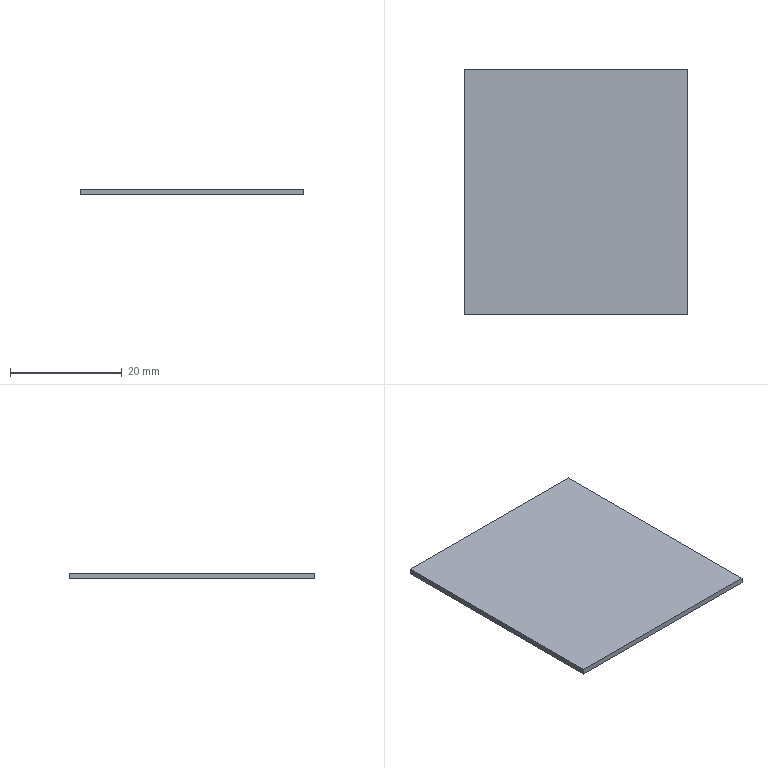Part | SolidWorks | features BaseBody 1 | 1 solid | 6 faces | box 40 x 44 x 1 mm | volume 1760 mm3 | plane 6
STEP:
#1=CARTESIAN_POINT('',(-20.,22.,0.));
#2=VERTEX_POINT('',#1);
#3=CARTESIAN_POINT('',(-20.,-22.,0.));
#4=VERTEX_POINT('',#3);
#5=CARTESIAN_POINT('',(-20.,22.,0.));
#6=DIRECTION('',(0.,-1.,0.));
#7=VECTOR('',#6,1000.);
#8=LINE('',#5,#7);
#9=EDGE_CURVE('',#2,#4,#8,.T.);
#10=ORIENTED_EDGE('',*,*,#9,.T.);
#11=CARTESIAN_POINT('',(-20.,-22.,1.));
#12=VERTEX_POINT('',#11);
#13=CARTESIAN_POINT('',(-20.,-22.,1.));
#14=DIRECTION('',(0.,0.,-1.));
#15=VECTOR('',#14,1000.);
#16=LINE('',#13,#15);
#17=EDGE_CURVE('',#12,#4,#16,.T.);
#18=ORIENTED_EDGE('',*,*,#17,.F.);
#19=CARTESIAN_POINT('',(-20.,22.,1.));
#20=VERTEX_POINT('',#19);
#21=CARTESIAN_POINT('',(-20.,22.,1.));
#22=DIRECTION('',(0.,-1.,0.));
#23=VECTOR('',#22,1000.);
#24=LINE('',#21,#23);
#25=EDGE_CURVE('',#20,#12,#24,.T.);
#26=ORIENTED_EDGE('',*,*,#25,.F.);
#27=CARTESIAN_POINT('',(-20.,22.,1.));
#28=DIRECTION('',(0.,0.,-1.));
#29=VECTOR('',#28,1000.);
#30=LINE('',#27,#29);
#31=EDGE_CURVE('',#20,#2,#30,.T.);
#32=ORIENTED_EDGE('',*,*,#31,.T.);
#33=EDGE_LOOP('',(#10,#18,#26,#32));
#34=FACE_OUTER_BOUND('',#33,.T.);
#35=CARTESIAN_POINT('',(-20.,22.,1.));
#36=DIRECTION('',(1.,0.,0.));
#37=DIRECTION('',(0.,1.,0.));
#38=AXIS2_PLACEMENT_3D('',#35,#36,#37);
#39=PLANE('',#38);
#40=ADVANCED_FACE('',(#34),#39,.F.);
#41=CARTESIAN_POINT('',(20.,-22.,0.));
#42=VERTEX_POINT('',#41);
#43=CARTESIAN_POINT('',(-20.,-22.,0.));
#44=DIRECTION('',(1.,0.,0.));
#45=VECTOR('',#44,1000.);
#46=LINE('',#43,#45);
#47=EDGE_CURVE('',#4,#42,#46,.T.);
#48=ORIENTED_EDGE('',*,*,#47,.T.);
#49=CARTESIAN_POINT('',(20.,-22.,1.));
#50=VERTEX_POINT('',#49);
#51=CARTESIAN_POINT('',(20.,-22.,1.));
#52=DIRECTION('',(0.,0.,-1.));
#53=VECTOR('',#52,1000.);
#54=LINE('',#51,#53);
#55=EDGE_CURVE('',#50,#42,#54,.T.);
#56=ORIENTED_EDGE('',*,*,#55,.F.);
#57=CARTESIAN_POINT('',(-20.,-22.,1.));
#58=DIRECTION('',(1.,0.,0.));
#59=VECTOR('',#58,1000.);
#60=LINE('',#57,#59);
#61=EDGE_CURVE('',#12,#50,#60,.T.);
#62=ORIENTED_EDGE('',*,*,#61,.F.);
#63=ORIENTED_EDGE('',*,*,#17,.T.);
#64=EDGE_LOOP('',(#48,#56,#62,#63));
#65=FACE_OUTER_BOUND('',#64,.T.);
#66=CARTESIAN_POINT('',(-20.,-22.,1.));
#67=DIRECTION('',(0.,1.,0.));
#68=DIRECTION('',(0.,0.,1.));
#69=AXIS2_PLACEMENT_3D('',#66,#67,#68);
#70=PLANE('',#69);
#71=ADVANCED_FACE('',(#65),#70,.F.);
#72=CARTESIAN_POINT('',(20.,22.,0.));
#73=VERTEX_POINT('',#72);
#74=CARTESIAN_POINT('',(20.,-22.,0.));
#75=DIRECTION('',(0.,1.,0.));
#76=VECTOR('',#75,1000.);
#77=LINE('',#74,#76);
#78=EDGE_CURVE('',#42,#73,#77,.T.);
#79=ORIENTED_EDGE('',*,*,#78,.T.);
#80=CARTESIAN_POINT('',(20.,22.,1.));
#81=VERTEX_POINT('',#80);
#82=CARTESIAN_POINT('',(20.,22.,1.));
#83=DIRECTION('',(0.,0.,-1.));
#84=VECTOR('',#83,1000.);
#85=LINE('',#82,#84);
#86=EDGE_CURVE('',#81,#73,#85,.T.);
#87=ORIENTED_EDGE('',*,*,#86,.F.);
#88=CARTESIAN_POINT('',(20.,-22.,1.));
#89=DIRECTION('',(0.,1.,0.));
#90=VECTOR('',#89,1000.);
#91=LINE('',#88,#90);
#92=EDGE_CURVE('',#50,#81,#91,.T.);
#93=ORIENTED_EDGE('',*,*,#92,.F.);
#94=ORIENTED_EDGE('',*,*,#55,.T.);
#95=EDGE_LOOP('',(#79,#87,#93,#94));
#96=FACE_OUTER_BOUND('',#95,.T.);
#97=CARTESIAN_POINT('',(20.,-22.,1.));
#98=DIRECTION('',(-1.,0.,0.));
#99=DIRECTION('',(0.,-1.,0.));
#100=AXIS2_PLACEMENT_3D('',#97,#98,#99);
#101=PLANE('',#100);
#102=ADVANCED_FACE('',(#96),#101,.F.);
#103=CARTESIAN_POINT('',(20.,22.,0.));
#104=DIRECTION('',(-1.,0.,0.));
#105=VECTOR('',#104,1000.);
#106=LINE('',#103,#105);
#107=EDGE_CURVE('',#73,#2,#106,.T.);
#108=ORIENTED_EDGE('',*,*,#107,.T.);
#109=ORIENTED_EDGE('',*,*,#31,.F.);
#110=CARTESIAN_POINT('',(20.,22.,1.));
#111=DIRECTION('',(-1.,0.,0.));
#112=VECTOR('',#111,1000.);
#113=LINE('',#110,#112);
#114=EDGE_CURVE('',#81,#20,#113,.T.);
#115=ORIENTED_EDGE('',*,*,#114,.F.);
#116=ORIENTED_EDGE('',*,*,#86,.T.);
#117=EDGE_LOOP('',(#108,#109,#115,#116));
#118=FACE_OUTER_BOUND('',#117,.T.);
#119=CARTESIAN_POINT('',(20.,22.,1.));
#120=DIRECTION('',(0.,-1.,0.));
#121=DIRECTION('',(0.,0.,-1.));
#122=AXIS2_PLACEMENT_3D('',#119,#120,#121);
#123=PLANE('',#122);
#124=ADVANCED_FACE('',(#118),#123,.F.);
#125=ORIENTED_EDGE('',*,*,#25,.T.);
#126=ORIENTED_EDGE('',*,*,#61,.T.);
#127=ORIENTED_EDGE('',*,*,#92,.T.);
#128=ORIENTED_EDGE('',*,*,#114,.T.);
#129=EDGE_LOOP('',(#125,#126,#127,#128));
#130=FACE_OUTER_BOUND('',#129,.T.);
#131=CARTESIAN_POINT('',(0.,0.,1.));
#132=DIRECTION('',(0.,0.,1.));
#133=DIRECTION('',(1.,0.,0.));
#134=AXIS2_PLACEMENT_3D('',#131,#132,#133);
#135=PLANE('',#134);
#136=ADVANCED_FACE('',(#130),#135,.T.);
#137=ORIENTED_EDGE('',*,*,#9,.F.);
#138=ORIENTED_EDGE('',*,*,#107,.F.);
#139=ORIENTED_EDGE('',*,*,#78,.F.);
#140=ORIENTED_EDGE('',*,*,#47,.F.);
#141=EDGE_LOOP('',(#137,#138,#139,#140));
#142=FACE_OUTER_BOUND('',#141,.T.);
#143=CARTESIAN_POINT('',(0.,0.,0.));
#144=DIRECTION('',(0.,0.,1.));
#145=DIRECTION('',(1.,0.,0.));
#146=AXIS2_PLACEMENT_3D('',#143,#144,#145);
#147=PLANE('',#146);
#148=ADVANCED_FACE('',(#142),#147,.F.);
#149=CLOSED_SHELL('',(#40,#71,#102,#124,#136,#148));
#150=MANIFOLD_SOLID_BREP('',#149);
#151=CARTESIAN_POINT('',(0.,0.,0.));
#152=DIRECTION('',(0.,0.,1.));
#153=DIRECTION('',(1.,0.,0.));
#154=AXIS2_PLACEMENT_3D('',#151,#152,#153);
#155=(LENGTH_UNIT()NAMED_UNIT(*)SI_UNIT(.MILLI.,.METRE.));
#156=UNCERTAINTY_MEASURE_WITH_UNIT(LENGTH_MEASURE(0.00001),#155,'','');
#157=(NAMED_UNIT(*)PLANE_ANGLE_UNIT()SI_UNIT($,.RADIAN.));
#158=(NAMED_UNIT(*)SI_UNIT($,.STERADIAN.)SOLID_ANGLE_UNIT());
#159=(GEOMETRIC_REPRESENTATION_CONTEXT(3)GLOBAL_UNCERTAINTY_ASSIGNED_CONTEXT((#156))GLOBAL_UNIT_ASSIGNED_CONTEXT((#155,#157,#158))REPRESENTATION_CONTEXT('',''));
#160=ADVANCED_BREP_SHAPE_REPRESENTATION('',(#150,#154),#159);